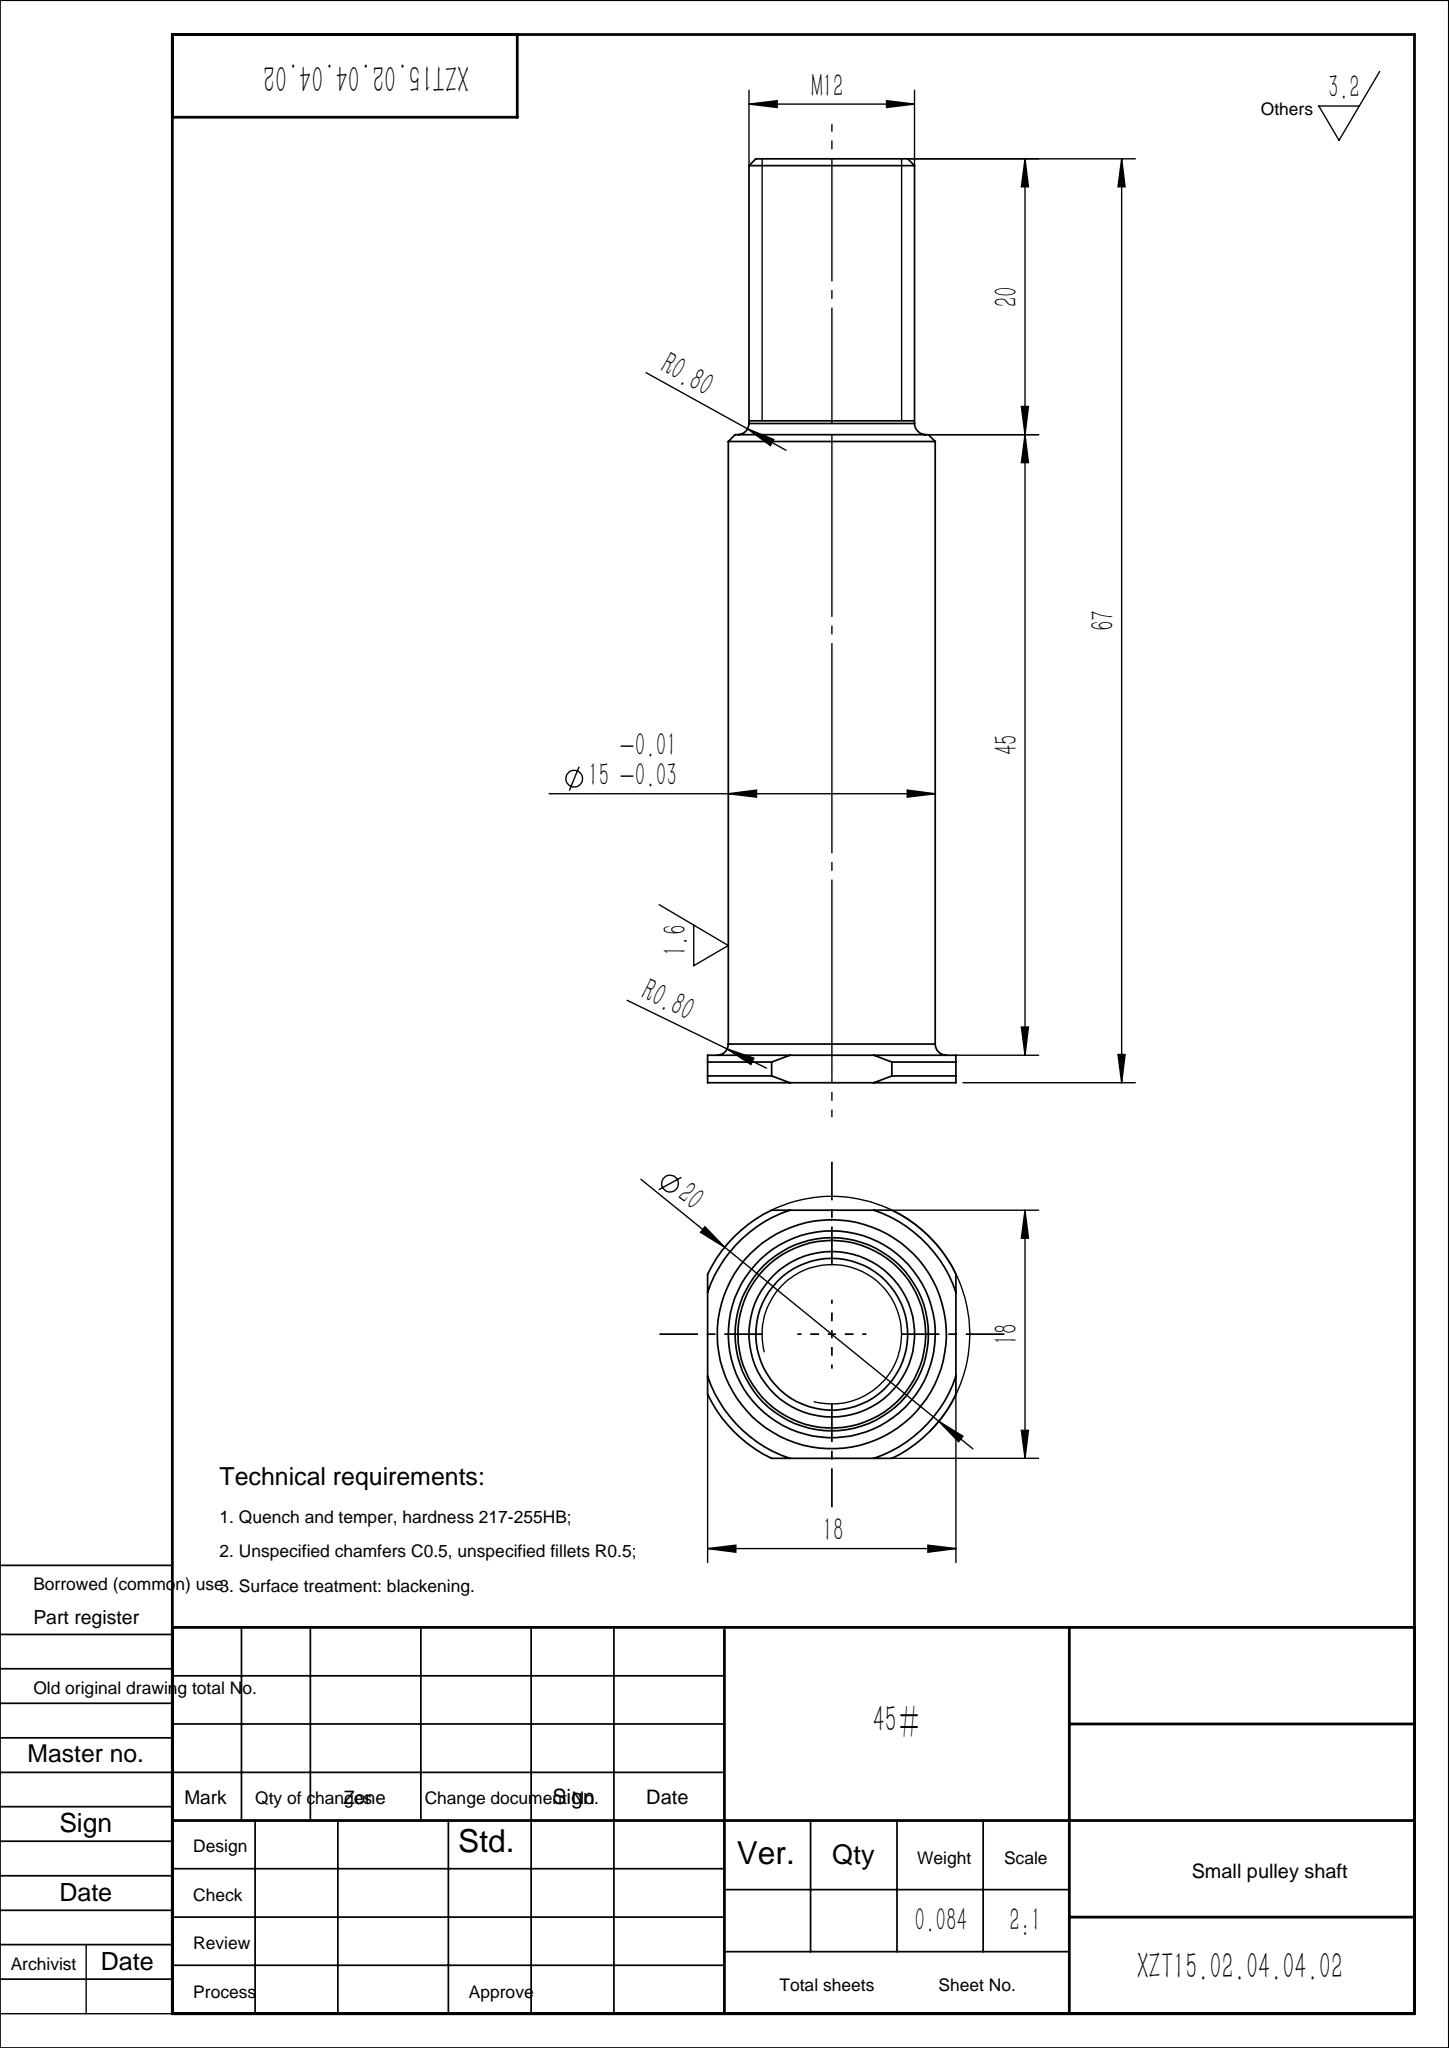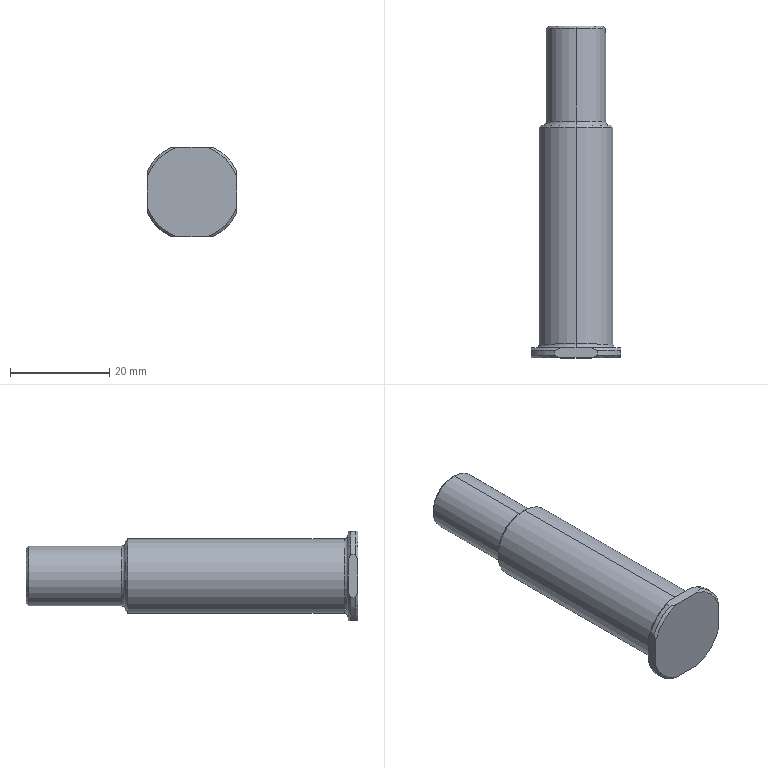Part | SolidWorks | features Chamfer 1, Fillet 1, ICE 1, Revolution 1 | 1 solid | 32 faces | box 18 x 67 x 18 mm | volume 10790 mm3 | cone 12 | cylinder 8 | plane 8 | torus 4 | commonest cylinder face diameters 20 x4 12 x2 15 x2
STEP:
#1=CARTESIAN_POINT('',(0.,2.,8.3));
#2=VERTEX_POINT('',#1);
#3=CARTESIAN_POINT('',(0.,2.,-8.3));
#4=VERTEX_POINT('',#3);
#5=CARTESIAN_POINT('',(0.,2.,0.));
#6=DIRECTION('',(0.,-1.,0.));
#7=DIRECTION('',(0.,0.,-1.));
#8=AXIS2_PLACEMENT_3D('',#5,#6,#7);
#9=CIRCLE('',#8,8.3);
#10=EDGE_CURVE('',#2,#4,#9,.T.);
#11=ORIENTED_EDGE('',*,*,#10,.F.);
#12=CARTESIAN_POINT('',(0.,2.8,7.5));
#13=VERTEX_POINT('',#12);
#14=CARTESIAN_POINT('',(0.,2.8,8.3));
#15=DIRECTION('',(1.,0.,0.));
#16=DIRECTION('',(0.,0.,-1.));
#17=AXIS2_PLACEMENT_3D('',#14,#15,#16);
#18=CIRCLE('',#17,0.8);
#19=EDGE_CURVE('',#2,#13,#18,.T.);
#20=ORIENTED_EDGE('',*,*,#19,.T.);
#21=CARTESIAN_POINT('',(0.,2.8,-7.5));
#22=VERTEX_POINT('',#21);
#23=CARTESIAN_POINT('',(0.,2.8,0.));
#24=DIRECTION('',(0.,1.,0.));
#25=DIRECTION('',(0.,0.,-1.));
#26=AXIS2_PLACEMENT_3D('',#23,#24,#25);
#27=CIRCLE('',#26,7.5);
#28=EDGE_CURVE('',#22,#13,#27,.T.);
#29=ORIENTED_EDGE('',*,*,#28,.F.);
#30=CARTESIAN_POINT('',(0.,2.8,-8.3));
#31=DIRECTION('',(-1.,0.,0.));
#32=DIRECTION('',(0.,0.,1.));
#33=AXIS2_PLACEMENT_3D('',#30,#31,#32);
#34=CIRCLE('',#33,0.8);
#35=EDGE_CURVE('',#4,#22,#34,.T.);
#36=ORIENTED_EDGE('',*,*,#35,.F.);
#37=EDGE_LOOP('',(#11,#20,#29,#36));
#38=FACE_OUTER_BOUND('',#37,.T.);
#39=CARTESIAN_POINT('',(0.,2.8,0.));
#40=DIRECTION('',(0.,-1.,0.));
#41=DIRECTION('',(0.,0.,-1.));
#42=AXIS2_PLACEMENT_3D('',#39,#40,#41);
#43=TOROIDAL_SURFACE('',#42,8.3,0.8);
#44=ADVANCED_FACE('',(#38),#43,.F.);
#45=CARTESIAN_POINT('',(0.,47.,6.8));
#46=VERTEX_POINT('',#45);
#47=CARTESIAN_POINT('',(0.,47.,-6.8));
#48=VERTEX_POINT('',#47);
#49=CARTESIAN_POINT('',(0.,47.,0.));
#50=DIRECTION('',(0.,-1.,0.));
#51=DIRECTION('',(0.,0.,-1.));
#52=AXIS2_PLACEMENT_3D('',#49,#50,#51);
#53=CIRCLE('',#52,6.8);
#54=EDGE_CURVE('',#46,#48,#53,.T.);
#55=ORIENTED_EDGE('',*,*,#54,.F.);
#56=CARTESIAN_POINT('',(0.,47.8,6.));
#57=VERTEX_POINT('',#56);
#58=CARTESIAN_POINT('',(0.,47.8,6.8));
#59=DIRECTION('',(1.,0.,0.));
#60=DIRECTION('',(0.,0.,-1.));
#61=AXIS2_PLACEMENT_3D('',#58,#59,#60);
#62=CIRCLE('',#61,0.8);
#63=EDGE_CURVE('',#46,#57,#62,.T.);
#64=ORIENTED_EDGE('',*,*,#63,.T.);
#65=CARTESIAN_POINT('',(0.,47.8,-6.));
#66=VERTEX_POINT('',#65);
#67=CARTESIAN_POINT('',(0.,47.8,0.));
#68=DIRECTION('',(0.,1.,0.));
#69=DIRECTION('',(0.,0.,-1.));
#70=AXIS2_PLACEMENT_3D('',#67,#68,#69);
#71=CIRCLE('',#70,6.);
#72=EDGE_CURVE('',#66,#57,#71,.T.);
#73=ORIENTED_EDGE('',*,*,#72,.F.);
#74=CARTESIAN_POINT('',(0.,47.8,-6.8));
#75=DIRECTION('',(-1.,0.,0.));
#76=DIRECTION('',(0.,0.,1.));
#77=AXIS2_PLACEMENT_3D('',#74,#75,#76);
#78=CIRCLE('',#77,0.8);
#79=EDGE_CURVE('',#48,#66,#78,.T.);
#80=ORIENTED_EDGE('',*,*,#79,.F.);
#81=EDGE_LOOP('',(#55,#64,#73,#80));
#82=FACE_OUTER_BOUND('',#81,.T.);
#83=CARTESIAN_POINT('',(0.,47.8,0.));
#84=DIRECTION('',(0.,-1.,0.));
#85=DIRECTION('',(0.,0.,-1.));
#86=AXIS2_PLACEMENT_3D('',#83,#84,#85);
#87=TOROIDAL_SURFACE('',#86,6.8,0.8);
#88=ADVANCED_FACE('',(#82),#87,.F.);
#89=CARTESIAN_POINT('',(0.,47.,7.));
#90=VERTEX_POINT('',#89);
#91=CARTESIAN_POINT('',(0.,47.,-7.));
#92=VERTEX_POINT('',#91);
#93=CARTESIAN_POINT('',(0.,47.,0.));
#94=DIRECTION('',(0.,1.,0.));
#95=DIRECTION('',(0.,0.,-1.));
#96=AXIS2_PLACEMENT_3D('',#93,#94,#95);
#97=CIRCLE('',#96,7.);
#98=EDGE_CURVE('',#90,#92,#97,.T.);
#99=ORIENTED_EDGE('',*,*,#98,.F.);
#100=CARTESIAN_POINT('',(0.,46.5,7.5));
#101=VERTEX_POINT('',#100);
#102=CARTESIAN_POINT('',(0.,47.,7.));
#103=DIRECTION('',(0.,-0.7071,0.7071));
#104=VECTOR('',#103,1000.);
#105=LINE('',#102,#104);
#106=EDGE_CURVE('',#90,#101,#105,.T.);
#107=ORIENTED_EDGE('',*,*,#106,.T.);
#108=CARTESIAN_POINT('',(0.,46.5,-7.5));
#109=VERTEX_POINT('',#108);
#110=CARTESIAN_POINT('',(0.,46.5,0.));
#111=DIRECTION('',(0.,-1.,0.));
#112=DIRECTION('',(0.,0.,-1.));
#113=AXIS2_PLACEMENT_3D('',#110,#111,#112);
#114=CIRCLE('',#113,7.5);
#115=EDGE_CURVE('',#109,#101,#114,.T.);
#116=ORIENTED_EDGE('',*,*,#115,.F.);
#117=CARTESIAN_POINT('',(0.,47.,-7.));
#118=DIRECTION('',(0.,-0.7071,-0.7071));
#119=VECTOR('',#118,1000.);
#120=LINE('',#117,#119);
#121=EDGE_CURVE('',#92,#109,#120,.T.);
#122=ORIENTED_EDGE('',*,*,#121,.F.);
#123=EDGE_LOOP('',(#99,#107,#116,#122));
#124=FACE_OUTER_BOUND('',#123,.T.);
#125=CARTESIAN_POINT('',(0.,47.,0.));
#126=DIRECTION('',(0.,-1.,0.));
#127=DIRECTION('',(0.,0.,-1.));
#128=AXIS2_PLACEMENT_3D('',#125,#126,#127);
#129=CONICAL_SURFACE('',#128,7.,0.7854);
#130=ADVANCED_FACE('',(#124),#129,.T.);
#131=CARTESIAN_POINT('',(0.,67.,5.5));
#132=VERTEX_POINT('',#131);
#133=CARTESIAN_POINT('',(0.,67.,-5.5));
#134=VERTEX_POINT('',#133);
#135=CARTESIAN_POINT('',(0.,67.,0.));
#136=DIRECTION('',(0.,1.,0.));
#137=DIRECTION('',(0.,0.,-1.));
#138=AXIS2_PLACEMENT_3D('',#135,#136,#137);
#139=CIRCLE('',#138,5.5);
#140=EDGE_CURVE('',#132,#134,#139,.T.);
#141=ORIENTED_EDGE('',*,*,#140,.F.);
#142=CARTESIAN_POINT('',(0.,66.5,6.));
#143=VERTEX_POINT('',#142);
#144=CARTESIAN_POINT('',(0.,67.,5.5));
#145=DIRECTION('',(0.,-0.7071,0.7071));
#146=VECTOR('',#145,1000.);
#147=LINE('',#144,#146);
#148=EDGE_CURVE('',#132,#143,#147,.T.);
#149=ORIENTED_EDGE('',*,*,#148,.T.);
#150=CARTESIAN_POINT('',(0.,66.5,-6.));
#151=VERTEX_POINT('',#150);
#152=CARTESIAN_POINT('',(0.,66.5,0.));
#153=DIRECTION('',(0.,-1.,0.));
#154=DIRECTION('',(0.,0.,-1.));
#155=AXIS2_PLACEMENT_3D('',#152,#153,#154);
#156=CIRCLE('',#155,6.);
#157=EDGE_CURVE('',#151,#143,#156,.T.);
#158=ORIENTED_EDGE('',*,*,#157,.F.);
#159=CARTESIAN_POINT('',(0.,67.,-5.5));
#160=DIRECTION('',(0.,-0.7071,-0.7071));
#161=VECTOR('',#160,1000.);
#162=LINE('',#159,#161);
#163=EDGE_CURVE('',#134,#151,#162,.T.);
#164=ORIENTED_EDGE('',*,*,#163,.F.);
#165=EDGE_LOOP('',(#141,#149,#158,#164));
#166=FACE_OUTER_BOUND('',#165,.T.);
#167=CARTESIAN_POINT('',(0.,67.,0.));
#168=DIRECTION('',(0.,-1.,0.));
#169=DIRECTION('',(0.,0.,-1.));
#170=AXIS2_PLACEMENT_3D('',#167,#168,#169);
#171=CONICAL_SURFACE('',#170,5.5,0.7854);
#172=ADVANCED_FACE('',(#166),#171,.T.);
#173=CARTESIAN_POINT('',(0.,47.8,0.));
#174=DIRECTION('',(0.,1.,0.));
#175=DIRECTION('',(0.,0.,-1.));
#176=AXIS2_PLACEMENT_3D('',#173,#174,#175);
#177=CIRCLE('',#176,6.);
#178=EDGE_CURVE('',#57,#66,#177,.T.);
#179=ORIENTED_EDGE('',*,*,#178,.T.);
#180=CARTESIAN_POINT('',(0.,0.,-6.));
#181=DIRECTION('',(0.,1.,0.));
#182=VECTOR('',#181,1000.);
#183=LINE('',#180,#182);
#184=EDGE_CURVE('',#66,#151,#183,.T.);
#185=ORIENTED_EDGE('',*,*,#184,.T.);
#186=ORIENTED_EDGE('',*,*,#157,.T.);
#187=CARTESIAN_POINT('',(0.,0.,6.));
#188=DIRECTION('',(0.,1.,0.));
#189=VECTOR('',#188,1000.);
#190=LINE('',#187,#189);
#191=EDGE_CURVE('',#57,#143,#190,.T.);
#192=ORIENTED_EDGE('',*,*,#191,.F.);
#193=EDGE_LOOP('',(#179,#185,#186,#192));
#194=FACE_OUTER_BOUND('',#193,.T.);
#195=CARTESIAN_POINT('',(0.,0.,0.));
#196=DIRECTION('',(0.,1.,0.));
#197=DIRECTION('',(0.,0.,1.));
#198=AXIS2_PLACEMENT_3D('',#195,#196,#197);
#199=CYLINDRICAL_SURFACE('',#198,6.);
#200=ADVANCED_FACE('',(#194),#199,.T.);
#201=CARTESIAN_POINT('',(0.,2.8,0.));
#202=DIRECTION('',(0.,1.,0.));
#203=DIRECTION('',(0.,0.,-1.));
#204=AXIS2_PLACEMENT_3D('',#201,#202,#203);
#205=CIRCLE('',#204,7.5);
#206=EDGE_CURVE('',#13,#22,#205,.T.);
#207=ORIENTED_EDGE('',*,*,#206,.T.);
#208=CARTESIAN_POINT('',(0.,0.,-7.5));
#209=DIRECTION('',(0.,1.,0.));
#210=VECTOR('',#209,1000.);
#211=LINE('',#208,#210);
#212=EDGE_CURVE('',#22,#109,#211,.T.);
#213=ORIENTED_EDGE('',*,*,#212,.T.);
#214=ORIENTED_EDGE('',*,*,#115,.T.);
#215=CARTESIAN_POINT('',(0.,0.,7.5));
#216=DIRECTION('',(0.,1.,0.));
#217=VECTOR('',#216,1000.);
#218=LINE('',#215,#217);
#219=EDGE_CURVE('',#13,#101,#218,.T.);
#220=ORIENTED_EDGE('',*,*,#219,.F.);
#221=EDGE_LOOP('',(#207,#213,#214,#220));
#222=FACE_OUTER_BOUND('',#221,.T.);
#223=CARTESIAN_POINT('',(0.,0.,0.));
#224=DIRECTION('',(0.,1.,0.));
#225=DIRECTION('',(0.,0.,1.));
#226=AXIS2_PLACEMENT_3D('',#223,#224,#225);
#227=CYLINDRICAL_SURFACE('',#226,7.5);
#228=ADVANCED_FACE('',(#222),#227,.T.);
#229=CARTESIAN_POINT('',(-4.359,0.5,-9.));
#230=VERTEX_POINT('',#229);
#231=CARTESIAN_POINT('',(-9.,0.5,-4.359));
#232=VERTEX_POINT('',#231);
#233=CARTESIAN_POINT('',(0.,0.5,0.));
#234=DIRECTION('',(0.,1.,0.));
#235=DIRECTION('',(0.,0.,1.));
#236=AXIS2_PLACEMENT_3D('',#233,#234,#235);
#237=CIRCLE('',#236,10.);
#238=EDGE_CURVE('',#230,#232,#237,.T.);
#239=ORIENTED_EDGE('',*,*,#238,.T.);
#240=CARTESIAN_POINT('',(-9.,1.5,-4.359));
#241=VERTEX_POINT('',#240);
#242=CARTESIAN_POINT('',(-9.,0.,-4.359));
#243=DIRECTION('',(0.,1.,0.));
#244=VECTOR('',#243,1000.);
#245=LINE('',#242,#244);
#246=EDGE_CURVE('',#232,#241,#245,.T.);
#247=ORIENTED_EDGE('',*,*,#246,.T.);
#248=CARTESIAN_POINT('',(-4.359,1.5,-9.));
#249=VERTEX_POINT('',#248);
#250=CARTESIAN_POINT('',(0.,1.5,0.));
#251=DIRECTION('',(0.,-1.,0.));
#252=DIRECTION('',(0.,0.,-1.));
#253=AXIS2_PLACEMENT_3D('',#250,#251,#252);
#254=CIRCLE('',#253,10.);
#255=EDGE_CURVE('',#241,#249,#254,.T.);
#256=ORIENTED_EDGE('',*,*,#255,.T.);
#257=CARTESIAN_POINT('',(-4.359,0.,-9.));
#258=DIRECTION('',(0.,-1.,0.));
#259=VECTOR('',#258,1000.);
#260=LINE('',#257,#259);
#261=EDGE_CURVE('',#249,#230,#260,.T.);
#262=ORIENTED_EDGE('',*,*,#261,.T.);
#263=EDGE_LOOP('',(#239,#247,#256,#262));
#264=FACE_OUTER_BOUND('',#263,.T.);
#265=CARTESIAN_POINT('',(0.,0.,0.));
#266=DIRECTION('',(0.,1.,0.));
#267=DIRECTION('',(0.,0.,1.));
#268=AXIS2_PLACEMENT_3D('',#265,#266,#267);
#269=CYLINDRICAL_SURFACE('',#268,10.);
#270=ADVANCED_FACE('',(#264),#269,.T.);
#271=CARTESIAN_POINT('',(-4.359,1.5,9.));
#272=VERTEX_POINT('',#271);
#273=CARTESIAN_POINT('',(-9.,1.5,4.359));
#274=VERTEX_POINT('',#273);
#275=CARTESIAN_POINT('',(0.,1.5,0.));
#276=DIRECTION('',(0.,-1.,0.));
#277=DIRECTION('',(0.,0.,-1.));
#278=AXIS2_PLACEMENT_3D('',#275,#276,#277);
#279=CIRCLE('',#278,10.);
#280=EDGE_CURVE('',#272,#274,#279,.T.);
#281=ORIENTED_EDGE('',*,*,#280,.T.);
#282=CARTESIAN_POINT('',(-9.,0.5,4.359));
#283=VERTEX_POINT('',#282);
#284=CARTESIAN_POINT('',(-9.,0.,4.359));
#285=DIRECTION('',(0.,-1.,0.));
#286=VECTOR('',#285,1000.);
#287=LINE('',#284,#286);
#288=EDGE_CURVE('',#274,#283,#287,.T.);
#289=ORIENTED_EDGE('',*,*,#288,.T.);
#290=CARTESIAN_POINT('',(-4.359,0.5,9.));
#291=VERTEX_POINT('',#290);
#292=CARTESIAN_POINT('',(0.,0.5,0.));
#293=DIRECTION('',(0.,1.,0.));
#294=DIRECTION('',(0.,0.,1.));
#295=AXIS2_PLACEMENT_3D('',#292,#293,#294);
#296=CIRCLE('',#295,10.);
#297=EDGE_CURVE('',#283,#291,#296,.T.);
#298=ORIENTED_EDGE('',*,*,#297,.T.);
#299=CARTESIAN_POINT('',(-4.359,0.,9.));
#300=DIRECTION('',(0.,1.,0.));
#301=VECTOR('',#300,1000.);
#302=LINE('',#299,#301);
#303=EDGE_CURVE('',#291,#272,#302,.T.);
#304=ORIENTED_EDGE('',*,*,#303,.T.);
#305=EDGE_LOOP('',(#281,#289,#298,#304));
#306=FACE_OUTER_BOUND('',#305,.T.);
#307=CARTESIAN_POINT('',(0.,0.,0.));
#308=DIRECTION('',(0.,1.,0.));
#309=DIRECTION('',(0.,0.,1.));
#310=AXIS2_PLACEMENT_3D('',#307,#308,#309);
#311=CYLINDRICAL_SURFACE('',#310,10.);
#312=ADVANCED_FACE('',(#306),#311,.T.);
#313=CARTESIAN_POINT('',(9.,1.5,4.359));
#314=VERTEX_POINT('',#313);
#315=CARTESIAN_POINT('',(4.359,1.5,9.));
#316=VERTEX_POINT('',#315);
#317=CARTESIAN_POINT('',(0.,1.5,0.));
#318=DIRECTION('',(0.,-1.,0.));
#319=DIRECTION('',(0.,0.,-1.));
#320=AXIS2_PLACEMENT_3D('',#317,#318,#319);
#321=CIRCLE('',#320,10.);
#322=EDGE_CURVE('',#314,#316,#321,.T.);
#323=ORIENTED_EDGE('',*,*,#322,.T.);
#324=CARTESIAN_POINT('',(4.359,0.5,9.));
#325=VERTEX_POINT('',#324);
#326=CARTESIAN_POINT('',(4.359,0.,9.));
#327=DIRECTION('',(0.,-1.,0.));
#328=VECTOR('',#327,1000.);
#329=LINE('',#326,#328);
#330=EDGE_CURVE('',#316,#325,#329,.T.);
#331=ORIENTED_EDGE('',*,*,#330,.T.);
#332=CARTESIAN_POINT('',(9.,0.5,4.359));
#333=VERTEX_POINT('',#332);
#334=CARTESIAN_POINT('',(0.,0.5,0.));
#335=DIRECTION('',(0.,1.,0.));
#336=DIRECTION('',(0.,0.,1.));
#337=AXIS2_PLACEMENT_3D('',#334,#335,#336);
#338=CIRCLE('',#337,10.);
#339=EDGE_CURVE('',#325,#333,#338,.T.);
#340=ORIENTED_EDGE('',*,*,#339,.T.);
#341=CARTESIAN_POINT('',(9.,0.,4.359));
#342=DIRECTION('',(0.,1.,0.));
#343=VECTOR('',#342,1000.);
#344=LINE('',#341,#343);
#345=EDGE_CURVE('',#333,#314,#344,.T.);
#346=ORIENTED_EDGE('',*,*,#345,.T.);
#347=EDGE_LOOP('',(#323,#331,#340,#346));
#348=FACE_OUTER_BOUND('',#347,.T.);
#349=CARTESIAN_POINT('',(0.,0.,0.));
#350=DIRECTION('',(0.,1.,0.));
#351=DIRECTION('',(0.,0.,1.));
#352=AXIS2_PLACEMENT_3D('',#349,#350,#351);
#353=CYLINDRICAL_SURFACE('',#352,10.);
#354=ADVANCED_FACE('',(#348),#353,.T.);
#355=CARTESIAN_POINT('',(-9.,2.,3.041));
#356=VERTEX_POINT('',#355);
#357=CARTESIAN_POINT('',(-9.,1.5,4.359));
#358=CARTESIAN_POINT('',(-9.,1.688,3.928));
#359=CARTESIAN_POINT('',(-9.,1.857,3.489));
#360=CARTESIAN_POINT('',(-9.,2.,3.041));
#361=B_SPLINE_CURVE_WITH_KNOTS('',3,(#357,#358,#359,#360),.UNSPECIFIED.,.F.,.F.,(4,4),(0.01807,0.01948),.UNSPECIFIED.);
#362=EDGE_CURVE('',#274,#356,#361,.T.);
#363=ORIENTED_EDGE('',*,*,#362,.F.);
#364=ORIENTED_EDGE('',*,*,#280,.F.);
#365=CARTESIAN_POINT('',(-3.041,2.,9.));
#366=VERTEX_POINT('',#365);
#367=CARTESIAN_POINT('',(-3.041,2.,9.));
#368=CARTESIAN_POINT('',(-3.488,1.857,9.));
#369=CARTESIAN_POINT('',(-3.927,1.688,9.));
#370=CARTESIAN_POINT('',(-4.359,1.5,9.));
#371=B_SPLINE_CURVE_WITH_KNOTS('',3,(#367,#368,#369,#370),.UNSPECIFIED.,.F.,.F.,(4,4),(0.02566,0.02708),.UNSPECIFIED.);
#372=EDGE_CURVE('',#366,#272,#371,.T.);
#373=ORIENTED_EDGE('',*,*,#372,.F.);
#374=CARTESIAN_POINT('',(0.,2.,0.));
#375=DIRECTION('',(0.,1.,0.));
#376=DIRECTION('',(0.,0.,-1.));
#377=AXIS2_PLACEMENT_3D('',#374,#375,#376);
#378=CIRCLE('',#377,9.5);
#379=EDGE_CURVE('',#356,#366,#378,.T.);
#380=ORIENTED_EDGE('',*,*,#379,.F.);
#381=EDGE_LOOP('',(#363,#364,#373,#380));
#382=FACE_OUTER_BOUND('',#381,.T.);
#383=CARTESIAN_POINT('',(0.,2.,0.));
#384=DIRECTION('',(0.,-1.,0.));
#385=DIRECTION('',(0.,0.,-1.));
#386=AXIS2_PLACEMENT_3D('',#383,#384,#385);
#387=CONICAL_SURFACE('',#386,9.5,0.7854);
#388=ADVANCED_FACE('',(#382),#387,.T.);
#389=CARTESIAN_POINT('',(3.041,2.,9.));
#390=VERTEX_POINT('',#389);
#391=CARTESIAN_POINT('',(4.359,1.5,9.));
#392=CARTESIAN_POINT('',(3.928,1.688,9.));
#393=CARTESIAN_POINT('',(3.489,1.857,9.));
#394=CARTESIAN_POINT('',(3.041,2.,9.));
#395=B_SPLINE_CURVE_WITH_KNOTS('',3,(#391,#392,#393,#394),.UNSPECIFIED.,.F.,.F.,(4,4),(0.01807,0.01948),.UNSPECIFIED.);
#396=EDGE_CURVE('',#316,#390,#395,.T.);
#397=ORIENTED_EDGE('',*,*,#396,.F.);
#398=ORIENTED_EDGE('',*,*,#322,.F.);
#399=CARTESIAN_POINT('',(9.,2.,3.041));
#400=VERTEX_POINT('',#399);
#401=CARTESIAN_POINT('',(9.,2.,3.041));
#402=CARTESIAN_POINT('',(9.,1.857,3.488));
#403=CARTESIAN_POINT('',(9.,1.688,3.927));
#404=CARTESIAN_POINT('',(9.,1.5,4.359));
#405=B_SPLINE_CURVE_WITH_KNOTS('',3,(#401,#402,#403,#404),.UNSPECIFIED.,.F.,.F.,(4,4),(0.02566,0.02708),.UNSPECIFIED.);
#406=EDGE_CURVE('',#400,#314,#405,.T.);
#407=ORIENTED_EDGE('',*,*,#406,.F.);
#408=CARTESIAN_POINT('',(0.,2.,0.));
#409=DIRECTION('',(0.,1.,0.));
#410=DIRECTION('',(0.,0.,-1.));
#411=AXIS2_PLACEMENT_3D('',#408,#409,#410);
#412=CIRCLE('',#411,9.5);
#413=EDGE_CURVE('',#390,#400,#412,.T.);
#414=ORIENTED_EDGE('',*,*,#413,.F.);
#415=EDGE_LOOP('',(#397,#398,#407,#414));
#416=FACE_OUTER_BOUND('',#415,.T.);
#417=CARTESIAN_POINT('',(0.,2.,0.));
#418=DIRECTION('',(0.,-1.,0.));
#419=DIRECTION('',(0.,0.,-1.));
#420=AXIS2_PLACEMENT_3D('',#417,#418,#419);
#421=CONICAL_SURFACE('',#420,9.5,0.7854);
#422=ADVANCED_FACE('',(#416),#421,.T.);
#423=CARTESIAN_POINT('',(9.,1.5,-4.359));
#424=VERTEX_POINT('',#423);
#425=CARTESIAN_POINT('',(9.,2.,-3.041));
#426=VERTEX_POINT('',#425);
#427=CARTESIAN_POINT('',(9.,1.5,-4.359));
#428=CARTESIAN_POINT('',(9.,1.688,-3.928));
#429=CARTESIAN_POINT('',(9.,1.857,-3.489));
#430=CARTESIAN_POINT('',(9.,2.,-3.041));
#431=B_SPLINE_CURVE_WITH_KNOTS('',3,(#427,#428,#429,#430),.UNSPECIFIED.,.F.,.F.,(4,4),(0.01807,0.01948),.UNSPECIFIED.);
#432=EDGE_CURVE('',#424,#426,#431,.T.);
#433=ORIENTED_EDGE('',*,*,#432,.F.);
#434=CARTESIAN_POINT('',(4.359,1.5,-9.));
#435=VERTEX_POINT('',#434);
#436=CARTESIAN_POINT('',(0.,1.5,0.));
#437=DIRECTION('',(0.,-1.,0.));
#438=DIRECTION('',(0.,0.,-1.));
#439=AXIS2_PLACEMENT_3D('',#436,#437,#438);
#440=CIRCLE('',#439,10.);
#441=EDGE_CURVE('',#435,#424,#440,.T.);
#442=ORIENTED_EDGE('',*,*,#441,.F.);
#443=CARTESIAN_POINT('',(3.041,2.,-9.));
#444=VERTEX_POINT('',#443);
#445=CARTESIAN_POINT('',(3.041,2.,-9.));
#446=CARTESIAN_POINT('',(3.488,1.857,-9.));
#447=CARTESIAN_POINT('',(3.927,1.688,-9.));
#448=CARTESIAN_POINT('',(4.359,1.5,-9.));
#449=B_SPLINE_CURVE_WITH_KNOTS('',3,(#445,#446,#447,#448),.UNSPECIFIED.,.F.,.F.,(4,4),(0.02566,0.02708),.UNSPECIFIED.);
#450=EDGE_CURVE('',#444,#435,#449,.T.);
#451=ORIENTED_EDGE('',*,*,#450,.F.);
#452=CARTESIAN_POINT('',(0.,2.,0.));
#453=DIRECTION('',(0.,1.,0.));
#454=DIRECTION('',(0.,0.,-1.));
#455=AXIS2_PLACEMENT_3D('',#452,#453,#454);
#456=CIRCLE('',#455,9.5);
#457=EDGE_CURVE('',#426,#444,#456,.T.);
#458=ORIENTED_EDGE('',*,*,#457,.F.);
#459=EDGE_LOOP('',(#433,#442,#451,#458));
#460=FACE_OUTER_BOUND('',#459,.T.);
#461=CARTESIAN_POINT('',(0.,2.,0.));
#462=DIRECTION('',(0.,-1.,0.));
#463=DIRECTION('',(0.,0.,-1.));
#464=AXIS2_PLACEMENT_3D('',#461,#462,#463);
#465=CONICAL_SURFACE('',#464,9.5,0.7854);
#466=ADVANCED_FACE('',(#460),#465,.T.);
#467=CARTESIAN_POINT('',(-9.,0.,-3.041));
#468=VERTEX_POINT('',#467);
#469=CARTESIAN_POINT('',(-9.,0.5,-4.359));
#470=CARTESIAN_POINT('',(-9.,0.312,-3.928));
#471=CARTESIAN_POINT('',(-9.,0.1434,-3.489));
#472=CARTESIAN_POINT('',(-9.,0.,-3.041));
#473=B_SPLINE_CURVE_WITH_KNOTS('',3,(#469,#470,#471,#472),.UNSPECIFIED.,.F.,.F.,(4,4),(0.01807,0.01948),.UNSPECIFIED.);
#474=EDGE_CURVE('',#232,#468,#473,.T.);
#475=ORIENTED_EDGE('',*,*,#474,.F.);
#476=ORIENTED_EDGE('',*,*,#238,.F.);
#477=CARTESIAN_POINT('',(-3.041,0.,-9.));
#478=VERTEX_POINT('',#477);
#479=CARTESIAN_POINT('',(-3.041,0.,-9.));
#480=CARTESIAN_POINT('',(-3.488,0.1431,-9.));
#481=CARTESIAN_POINT('',(-3.927,0.3117,-9.));
#482=CARTESIAN_POINT('',(-4.359,0.5,-9.));
#483=B_SPLINE_CURVE_WITH_KNOTS('',3,(#479,#480,#481,#482),.UNSPECIFIED.,.F.,.F.,(4,4),(0.02566,0.02708),.UNSPECIFIED.);
#484=EDGE_CURVE('',#478,#230,#483,.T.);
#485=ORIENTED_EDGE('',*,*,#484,.F.);
#486=CARTESIAN_POINT('',(0.,0.,0.));
#487=DIRECTION('',(0.,-1.,0.));
#488=DIRECTION('',(0.,0.,1.));
#489=AXIS2_PLACEMENT_3D('',#486,#487,#488);
#490=CIRCLE('',#489,9.5);
#491=EDGE_CURVE('',#468,#478,#490,.T.);
#492=ORIENTED_EDGE('',*,*,#491,.F.);
#493=EDGE_LOOP('',(#475,#476,#485,#492));
#494=FACE_OUTER_BOUND('',#493,.T.);
#495=CARTESIAN_POINT('',(0.,0.5,0.));
#496=DIRECTION('',(0.,1.,0.));
#497=DIRECTION('',(0.,0.,1.));
#498=AXIS2_PLACEMENT_3D('',#495,#496,#497);
#499=CONICAL_SURFACE('',#498,10.,0.7854);
#500=ADVANCED_FACE('',(#494),#499,.T.);
#501=CARTESIAN_POINT('',(-9.,0.,3.041));
#502=VERTEX_POINT('',#501);
#503=CARTESIAN_POINT('',(-9.,0.,3.041));
#504=CARTESIAN_POINT('',(-9.,0.1431,3.488));
#505=CARTESIAN_POINT('',(-9.,0.3117,3.927));
#506=CARTESIAN_POINT('',(-9.,0.5,4.359));
#507=B_SPLINE_CURVE_WITH_KNOTS('',3,(#503,#504,#505,#506),.UNSPECIFIED.,.F.,.F.,(4,4),(0.02566,0.02708),.UNSPECIFIED.);
#508=EDGE_CURVE('',#502,#283,#507,.T.);
#509=ORIENTED_EDGE('',*,*,#508,.F.);
#510=CARTESIAN_POINT('',(-3.041,0.,9.));
#511=VERTEX_POINT('',#510);
#512=CARTESIAN_POINT('',(0.,0.,0.));
#513=DIRECTION('',(0.,-1.,0.));
#514=DIRECTION('',(0.,0.,1.));
#515=AXIS2_PLACEMENT_3D('',#512,#513,#514);
#516=CIRCLE('',#515,9.5);
#517=EDGE_CURVE('',#511,#502,#516,.T.);
#518=ORIENTED_EDGE('',*,*,#517,.F.);
#519=CARTESIAN_POINT('',(-4.359,0.5,9.));
#520=CARTESIAN_POINT('',(-3.928,0.312,9.));
#521=CARTESIAN_POINT('',(-3.489,0.1434,9.));
#522=CARTESIAN_POINT('',(-3.041,0.,9.));
#523=B_SPLINE_CURVE_WITH_KNOTS('',3,(#519,#520,#521,#522),.UNSPECIFIED.,.F.,.F.,(4,4),(0.01807,0.01948),.UNSPECIFIED.);
#524=EDGE_CURVE('',#291,#511,#523,.T.);
#525=ORIENTED_EDGE('',*,*,#524,.F.);
#526=ORIENTED_EDGE('',*,*,#297,.F.);
#527=EDGE_LOOP('',(#509,#518,#525,#526));
#528=FACE_OUTER_BOUND('',#527,.T.);
#529=CARTESIAN_POINT('',(0.,0.5,0.));
#530=DIRECTION('',(0.,1.,0.));
#531=DIRECTION('',(0.,0.,1.));
#532=AXIS2_PLACEMENT_3D('',#529,#530,#531);
#533=CONICAL_SURFACE('',#532,10.,0.7854);
#534=ADVANCED_FACE('',(#528),#533,.T.);
#535=CARTESIAN_POINT('',(3.041,0.,9.));
#536=VERTEX_POINT('',#535);
#537=CARTESIAN_POINT('',(3.041,0.,9.));
#538=CARTESIAN_POINT('',(3.488,0.1431,9.));
#539=CARTESIAN_POINT('',(3.927,0.3117,9.));
#540=CARTESIAN_POINT('',(4.359,0.5,9.));
#541=B_SPLINE_CURVE_WITH_KNOTS('',3,(#537,#538,#539,#540),.UNSPECIFIED.,.F.,.F.,(4,4),(0.02566,0.02708),.UNSPECIFIED.);
#542=EDGE_CURVE('',#536,#325,#541,.T.);
#543=ORIENTED_EDGE('',*,*,#542,.F.);
#544=CARTESIAN_POINT('',(9.,0.,3.041));
#545=VERTEX_POINT('',#544);
#546=CARTESIAN_POINT('',(0.,0.,0.));
#547=DIRECTION('',(0.,-1.,0.));
#548=DIRECTION('',(0.,0.,1.));
#549=AXIS2_PLACEMENT_3D('',#546,#547,#548);
#550=CIRCLE('',#549,9.5);
#551=EDGE_CURVE('',#545,#536,#550,.T.);
#552=ORIENTED_EDGE('',*,*,#551,.F.);
#553=CARTESIAN_POINT('',(9.,0.5,4.359));
#554=CARTESIAN_POINT('',(9.,0.312,3.928));
#555=CARTESIAN_POINT('',(9.,0.1434,3.489));
#556=CARTESIAN_POINT('',(9.,0.,3.041));
#557=B_SPLINE_CURVE_WITH_KNOTS('',3,(#553,#554,#555,#556),.UNSPECIFIED.,.F.,.F.,(4,4),(0.01807,0.01948),.UNSPECIFIED.);
#558=EDGE_CURVE('',#333,#545,#557,.T.);
#559=ORIENTED_EDGE('',*,*,#558,.F.);
#560=ORIENTED_EDGE('',*,*,#339,.F.);
#561=EDGE_LOOP('',(#543,#552,#559,#560));
#562=FACE_OUTER_BOUND('',#561,.T.);
#563=CARTESIAN_POINT('',(0.,0.5,0.));
#564=DIRECTION('',(0.,1.,0.));
#565=DIRECTION('',(0.,0.,1.));
#566=AXIS2_PLACEMENT_3D('',#563,#564,#565);
#567=CONICAL_SURFACE('',#566,10.,0.7854);
#568=ADVANCED_FACE('',(#562),#567,.T.);
#569=ORIENTED_EDGE('',*,*,#517,.T.);
#570=CARTESIAN_POINT('',(-9.,0.,9.));
#571=DIRECTION('',(0.,0.,1.));
#572=VECTOR('',#571,1000.);
#573=LINE('',#570,#572);
#574=EDGE_CURVE('',#468,#502,#573,.T.);
#575=ORIENTED_EDGE('',*,*,#574,.F.);
#576=ORIENTED_EDGE('',*,*,#491,.T.);
#577=CARTESIAN_POINT('',(3.041,0.,-9.));
#578=VERTEX_POINT('',#577);
#579=CARTESIAN_POINT('',(9.,0.,-9.));
#580=DIRECTION('',(-1.,0.,0.));
#581=VECTOR('',#580,1000.);
#582=LINE('',#579,#581);
#583=EDGE_CURVE('',#578,#478,#582,.T.);
#584=ORIENTED_EDGE('',*,*,#583,.F.);
#585=CARTESIAN_POINT('',(9.,0.,-3.041));
#586=VERTEX_POINT('',#585);
#587=CARTESIAN_POINT('',(0.,0.,0.));
#588=DIRECTION('',(0.,-1.,0.));
#589=DIRECTION('',(0.,0.,1.));
#590=AXIS2_PLACEMENT_3D('',#587,#588,#589);
#591=CIRCLE('',#590,9.5);
#592=EDGE_CURVE('',#578,#586,#591,.T.);
#593=ORIENTED_EDGE('',*,*,#592,.T.);
#594=CARTESIAN_POINT('',(9.,0.,9.));
#595=DIRECTION('',(0.,0.,-1.));
#596=VECTOR('',#595,1000.);
#597=LINE('',#594,#596);
#598=EDGE_CURVE('',#545,#586,#597,.T.);
#599=ORIENTED_EDGE('',*,*,#598,.F.);
#600=ORIENTED_EDGE('',*,*,#551,.T.);
#601=CARTESIAN_POINT('',(9.,0.,9.));
#602=DIRECTION('',(1.,0.,0.));
#603=VECTOR('',#602,1000.);
#604=LINE('',#601,#603);
#605=EDGE_CURVE('',#511,#536,#604,.T.);
#606=ORIENTED_EDGE('',*,*,#605,.F.);
#607=EDGE_LOOP('',(#569,#575,#576,#584,#593,#599,#600,#606));
#608=FACE_OUTER_BOUND('',#607,.T.);
#609=CARTESIAN_POINT('',(0.,0.,0.));
#610=DIRECTION('',(0.,1.,0.));
#611=DIRECTION('',(0.,0.,1.));
#612=AXIS2_PLACEMENT_3D('',#609,#610,#611);
#613=PLANE('',#612);
#614=ADVANCED_FACE('',(#608),#613,.F.);
#615=ORIENTED_EDGE('',*,*,#441,.T.);
#616=CARTESIAN_POINT('',(9.,0.5,-4.359));
#617=VERTEX_POINT('',#616);
#618=CARTESIAN_POINT('',(9.,0.,-4.359));
#619=DIRECTION('',(0.,-1.,0.));
#620=VECTOR('',#619,1000.);
#621=LINE('',#618,#620);
#622=EDGE_CURVE('',#424,#617,#621,.T.);
#623=ORIENTED_EDGE('',*,*,#622,.T.);
#624=CARTESIAN_POINT('',(4.359,0.5,-9.));
#625=VERTEX_POINT('',#624);
#626=CARTESIAN_POINT('',(0.,0.5,0.));
#627=DIRECTION('',(0.,1.,0.));
#628=DIRECTION('',(0.,0.,1.));
#629=AXIS2_PLACEMENT_3D('',#626,#627,#628);
#630=CIRCLE('',#629,10.);
#631=EDGE_CURVE('',#617,#625,#630,.T.);
#632=ORIENTED_EDGE('',*,*,#631,.T.);
#633=CARTESIAN_POINT('',(4.359,0.,-9.));
#634=DIRECTION('',(0.,1.,0.));
#635=VECTOR('',#634,1000.);
#636=LINE('',#633,#635);
#637=EDGE_CURVE('',#625,#435,#636,.T.);
#638=ORIENTED_EDGE('',*,*,#637,.T.);
#639=EDGE_LOOP('',(#615,#623,#632,#638));
#640=FACE_OUTER_BOUND('',#639,.T.);
#641=CARTESIAN_POINT('',(0.,0.,0.));
#642=DIRECTION('',(0.,1.,0.));
#643=DIRECTION('',(0.,0.,1.));
#644=AXIS2_PLACEMENT_3D('',#641,#642,#643);
#645=CYLINDRICAL_SURFACE('',#644,10.);
#646=ADVANCED_FACE('',(#640),#645,.T.);
#647=CARTESIAN_POINT('',(0.,2.,0.));
#648=DIRECTION('',(0.,-1.,0.));
#649=DIRECTION('',(0.,0.,-1.));
#650=AXIS2_PLACEMENT_3D('',#647,#648,#649);
#651=CIRCLE('',#650,8.3);
#652=EDGE_CURVE('',#4,#2,#651,.T.);
#653=ORIENTED_EDGE('',*,*,#652,.T.);
#654=ORIENTED_EDGE('',*,*,#10,.T.);
#655=EDGE_LOOP('',(#653,#654));
#656=FACE_BOUND('',#655,.T.);
#657=CARTESIAN_POINT('',(-3.041,2.,-9.));
#658=VERTEX_POINT('',#657);
#659=CARTESIAN_POINT('',(-9.,2.,-3.041));
#660=VERTEX_POINT('',#659);
#661=CARTESIAN_POINT('',(0.,2.,0.));
#662=DIRECTION('',(0.,1.,0.));
#663=DIRECTION('',(0.,0.,-1.));
#664=AXIS2_PLACEMENT_3D('',#661,#662,#663);
#665=CIRCLE('',#664,9.5);
#666=EDGE_CURVE('',#658,#660,#665,.T.);
#667=ORIENTED_EDGE('',*,*,#666,.T.);
#668=CARTESIAN_POINT('',(-9.,2.,0.));
#669=DIRECTION('',(0.,0.,1.));
#670=VECTOR('',#669,1000.);
#671=LINE('',#668,#670);
#672=EDGE_CURVE('',#660,#356,#671,.T.);
#673=ORIENTED_EDGE('',*,*,#672,.T.);
#674=ORIENTED_EDGE('',*,*,#379,.T.);
#675=CARTESIAN_POINT('',(10.,2.,9.));
#676=DIRECTION('',(1.,0.,0.));
#677=VECTOR('',#676,1000.);
#678=LINE('',#675,#677);
#679=EDGE_CURVE('',#366,#390,#678,.T.);
#680=ORIENTED_EDGE('',*,*,#679,.T.);
#681=ORIENTED_EDGE('',*,*,#413,.T.);
#682=CARTESIAN_POINT('',(9.,2.,0.));
#683=DIRECTION('',(0.,0.,-1.));
#684=VECTOR('',#683,1000.);
#685=LINE('',#682,#684);
#686=EDGE_CURVE('',#400,#426,#685,.T.);
#687=ORIENTED_EDGE('',*,*,#686,.T.);
#688=ORIENTED_EDGE('',*,*,#457,.T.);
#689=CARTESIAN_POINT('',(10.,2.,-9.));
#690=DIRECTION('',(-1.,0.,0.));
#691=VECTOR('',#690,1000.);
#692=LINE('',#689,#691);
#693=EDGE_CURVE('',#444,#658,#692,.T.);
#694=ORIENTED_EDGE('',*,*,#693,.T.);
#695=EDGE_LOOP('',(#667,#673,#674,#680,#681,#687,#688,#694));
#696=FACE_OUTER_BOUND('',#695,.T.);
#697=CARTESIAN_POINT('',(10.,2.,0.));
#698=DIRECTION('',(0.,-1.,0.));
#699=DIRECTION('',(0.,0.,-1.));
#700=AXIS2_PLACEMENT_3D('',#697,#698,#699);
#701=PLANE('',#700);
#702=ADVANCED_FACE('',(#656,#696),#701,.F.);
#703=ORIENTED_EDGE('',*,*,#212,.F.);
#704=ORIENTED_EDGE('',*,*,#28,.T.);
#705=ORIENTED_EDGE('',*,*,#219,.T.);
#706=CARTESIAN_POINT('',(0.,46.5,0.));
#707=DIRECTION('',(0.,-1.,0.));
#708=DIRECTION('',(0.,0.,-1.));
#709=AXIS2_PLACEMENT_3D('',#706,#707,#708);
#710=CIRCLE('',#709,7.5);
#711=EDGE_CURVE('',#101,#109,#710,.T.);
#712=ORIENTED_EDGE('',*,*,#711,.T.);
#713=EDGE_LOOP('',(#703,#704,#705,#712));
#714=FACE_OUTER_BOUND('',#713,.T.);
#715=CARTESIAN_POINT('',(0.,0.,0.));
#716=DIRECTION('',(0.,1.,0.));
#717=DIRECTION('',(0.,0.,1.));
#718=AXIS2_PLACEMENT_3D('',#715,#716,#717);
#719=CYLINDRICAL_SURFACE('',#718,7.5);
#720=ADVANCED_FACE('',(#714),#719,.T.);
#721=CARTESIAN_POINT('',(0.,47.,0.));
#722=DIRECTION('',(0.,-1.,0.));
#723=DIRECTION('',(0.,0.,-1.));
#724=AXIS2_PLACEMENT_3D('',#721,#722,#723);
#725=CIRCLE('',#724,6.8);
#726=EDGE_CURVE('',#48,#46,#725,.T.);
#727=ORIENTED_EDGE('',*,*,#726,.T.);
#728=ORIENTED_EDGE('',*,*,#54,.T.);
#729=EDGE_LOOP('',(#727,#728));
#730=FACE_BOUND('',#729,.T.);
#731=CARTESIAN_POINT('',(0.,47.,0.));
#732=DIRECTION('',(0.,1.,0.));
#733=DIRECTION('',(0.,0.,-1.));
#734=AXIS2_PLACEMENT_3D('',#731,#732,#733);
#735=CIRCLE('',#734,7.);
#736=EDGE_CURVE('',#92,#90,#735,.T.);
#737=ORIENTED_EDGE('',*,*,#736,.T.);
#738=ORIENTED_EDGE('',*,*,#98,.T.);
#739=EDGE_LOOP('',(#737,#738));
#740=FACE_OUTER_BOUND('',#739,.T.);
#741=CARTESIAN_POINT('',(7.5,47.,0.));
#742=DIRECTION('',(0.,-1.,0.));
#743=DIRECTION('',(0.,0.,-1.));
#744=AXIS2_PLACEMENT_3D('',#741,#742,#743);
#745=PLANE('',#744);
#746=ADVANCED_FACE('',(#730,#740),#745,.F.);
#747=ORIENTED_EDGE('',*,*,#184,.F.);
#748=ORIENTED_EDGE('',*,*,#72,.T.);
#749=ORIENTED_EDGE('',*,*,#191,.T.);
#750=CARTESIAN_POINT('',(0.,66.5,0.));
#751=DIRECTION('',(0.,-1.,0.));
#752=DIRECTION('',(0.,0.,-1.));
#753=AXIS2_PLACEMENT_3D('',#750,#751,#752);
#754=CIRCLE('',#753,6.);
#755=EDGE_CURVE('',#143,#151,#754,.T.);
#756=ORIENTED_EDGE('',*,*,#755,.T.);
#757=EDGE_LOOP('',(#747,#748,#749,#756));
#758=FACE_OUTER_BOUND('',#757,.T.);
#759=CARTESIAN_POINT('',(0.,0.,0.));
#760=DIRECTION('',(0.,1.,0.));
#761=DIRECTION('',(0.,0.,1.));
#762=AXIS2_PLACEMENT_3D('',#759,#760,#761);
#763=CYLINDRICAL_SURFACE('',#762,6.);
#764=ADVANCED_FACE('',(#758),#763,.T.);
#765=CARTESIAN_POINT('',(0.,67.,0.));
#766=DIRECTION('',(0.,1.,0.));
#767=DIRECTION('',(0.,0.,-1.));
#768=AXIS2_PLACEMENT_3D('',#765,#766,#767);
#769=CIRCLE('',#768,5.5);
#770=EDGE_CURVE('',#134,#132,#769,.T.);
#771=ORIENTED_EDGE('',*,*,#770,.T.);
#772=ORIENTED_EDGE('',*,*,#140,.T.);
#773=EDGE_LOOP('',(#771,#772));
#774=FACE_OUTER_BOUND('',#773,.T.);
#775=CARTESIAN_POINT('',(6.,67.,0.));
#776=DIRECTION('',(0.,-1.,0.));
#777=DIRECTION('',(0.,0.,-1.));
#778=AXIS2_PLACEMENT_3D('',#775,#776,#777);
#779=PLANE('',#778);
#780=ADVANCED_FACE('',(#774),#779,.F.);
#781=ORIENTED_EDGE('',*,*,#148,.F.);
#782=ORIENTED_EDGE('',*,*,#770,.F.);
#783=ORIENTED_EDGE('',*,*,#163,.T.);
#784=ORIENTED_EDGE('',*,*,#755,.F.);
#785=EDGE_LOOP('',(#781,#782,#783,#784));
#786=FACE_OUTER_BOUND('',#785,.T.);
#787=CARTESIAN_POINT('',(0.,67.,0.));
#788=DIRECTION('',(0.,-1.,0.));
#789=DIRECTION('',(0.,0.,-1.));
#790=AXIS2_PLACEMENT_3D('',#787,#788,#789);
#791=CONICAL_SURFACE('',#790,5.5,0.7854);
#792=ADVANCED_FACE('',(#786),#791,.T.);
#793=CARTESIAN_POINT('',(-9.,2.,-3.041));
#794=CARTESIAN_POINT('',(-9.,1.857,-3.488));
#795=CARTESIAN_POINT('',(-9.,1.688,-3.927));
#796=CARTESIAN_POINT('',(-9.,1.5,-4.359));
#797=B_SPLINE_CURVE_WITH_KNOTS('',3,(#793,#794,#795,#796),.UNSPECIFIED.,.F.,.F.,(4,4),(0.02566,0.02708),.UNSPECIFIED.);
#798=EDGE_CURVE('',#660,#241,#797,.T.);
#799=ORIENTED_EDGE('',*,*,#798,.F.);
#800=ORIENTED_EDGE('',*,*,#666,.F.);
#801=CARTESIAN_POINT('',(-4.359,1.5,-9.));
#802=CARTESIAN_POINT('',(-3.928,1.688,-9.));
#803=CARTESIAN_POINT('',(-3.489,1.857,-9.));
#804=CARTESIAN_POINT('',(-3.041,2.,-9.));
#805=B_SPLINE_CURVE_WITH_KNOTS('',3,(#801,#802,#803,#804),.UNSPECIFIED.,.F.,.F.,(4,4),(0.01807,0.01948),.UNSPECIFIED.);
#806=EDGE_CURVE('',#249,#658,#805,.T.);
#807=ORIENTED_EDGE('',*,*,#806,.F.);
#808=ORIENTED_EDGE('',*,*,#255,.F.);
#809=EDGE_LOOP('',(#799,#800,#807,#808));
#810=FACE_OUTER_BOUND('',#809,.T.);
#811=CARTESIAN_POINT('',(0.,2.,0.));
#812=DIRECTION('',(0.,-1.,0.));
#813=DIRECTION('',(0.,0.,-1.));
#814=AXIS2_PLACEMENT_3D('',#811,#812,#813);
#815=CONICAL_SURFACE('',#814,9.5,0.7854);
#816=ADVANCED_FACE('',(#810),#815,.T.);
#817=CARTESIAN_POINT('',(9.,0.,-3.041));
#818=CARTESIAN_POINT('',(9.,0.1431,-3.488));
#819=CARTESIAN_POINT('',(9.,0.3117,-3.927));
#820=CARTESIAN_POINT('',(9.,0.5,-4.359));
#821=B_SPLINE_CURVE_WITH_KNOTS('',3,(#817,#818,#819,#820),.UNSPECIFIED.,.F.,.F.,(4,4),(0.02566,0.02708),.UNSPECIFIED.);
#822=EDGE_CURVE('',#586,#617,#821,.T.);
#823=ORIENTED_EDGE('',*,*,#822,.F.);
#824=ORIENTED_EDGE('',*,*,#592,.F.);
#825=CARTESIAN_POINT('',(4.359,0.5,-9.));
#826=CARTESIAN_POINT('',(3.928,0.312,-9.));
#827=CARTESIAN_POINT('',(3.489,0.1434,-9.));
#828=CARTESIAN_POINT('',(3.041,0.,-9.));
#829=B_SPLINE_CURVE_WITH_KNOTS('',3,(#825,#826,#827,#828),.UNSPECIFIED.,.F.,.F.,(4,4),(0.01807,0.01948),.UNSPECIFIED.);
#830=EDGE_CURVE('',#625,#578,#829,.T.);
#831=ORIENTED_EDGE('',*,*,#830,.F.);
#832=ORIENTED_EDGE('',*,*,#631,.F.);
#833=EDGE_LOOP('',(#823,#824,#831,#832));
#834=FACE_OUTER_BOUND('',#833,.T.);
#835=CARTESIAN_POINT('',(0.,0.5,0.));
#836=DIRECTION('',(0.,1.,0.));
#837=DIRECTION('',(0.,0.,1.));
#838=AXIS2_PLACEMENT_3D('',#835,#836,#837);
#839=CONICAL_SURFACE('',#838,10.,0.7854);
#840=ADVANCED_FACE('',(#834),#839,.T.);
#841=ORIENTED_EDGE('',*,*,#106,.F.);
#842=ORIENTED_EDGE('',*,*,#736,.F.);
#843=ORIENTED_EDGE('',*,*,#121,.T.);
#844=ORIENTED_EDGE('',*,*,#711,.F.);
#845=EDGE_LOOP('',(#841,#842,#843,#844));
#846=FACE_OUTER_BOUND('',#845,.T.);
#847=CARTESIAN_POINT('',(0.,47.,0.));
#848=DIRECTION('',(0.,-1.,0.));
#849=DIRECTION('',(0.,0.,-1.));
#850=AXIS2_PLACEMENT_3D('',#847,#848,#849);
#851=CONICAL_SURFACE('',#850,7.,0.7854);
#852=ADVANCED_FACE('',(#846),#851,.T.);
#853=ORIENTED_EDGE('',*,*,#63,.F.);
#854=ORIENTED_EDGE('',*,*,#726,.F.);
#855=ORIENTED_EDGE('',*,*,#79,.T.);
#856=ORIENTED_EDGE('',*,*,#178,.F.);
#857=EDGE_LOOP('',(#853,#854,#855,#856));
#858=FACE_OUTER_BOUND('',#857,.T.);
#859=CARTESIAN_POINT('',(0.,47.8,0.));
#860=DIRECTION('',(0.,-1.,0.));
#861=DIRECTION('',(0.,0.,-1.));
#862=AXIS2_PLACEMENT_3D('',#859,#860,#861);
#863=TOROIDAL_SURFACE('',#862,6.8,0.8);
#864=ADVANCED_FACE('',(#858),#863,.F.);
#865=ORIENTED_EDGE('',*,*,#19,.F.);
#866=ORIENTED_EDGE('',*,*,#652,.F.);
#867=ORIENTED_EDGE('',*,*,#35,.T.);
#868=ORIENTED_EDGE('',*,*,#206,.F.);
#869=EDGE_LOOP('',(#865,#866,#867,#868));
#870=FACE_OUTER_BOUND('',#869,.T.);
#871=CARTESIAN_POINT('',(0.,2.8,0.));
#872=DIRECTION('',(0.,-1.,0.));
#873=DIRECTION('',(0.,0.,-1.));
#874=AXIS2_PLACEMENT_3D('',#871,#872,#873);
#875=TOROIDAL_SURFACE('',#874,8.3,0.8);
#876=ADVANCED_FACE('',(#870),#875,.F.);
#877=ORIENTED_EDGE('',*,*,#830,.T.);
#878=ORIENTED_EDGE('',*,*,#583,.T.);
#879=ORIENTED_EDGE('',*,*,#484,.T.);
#880=ORIENTED_EDGE('',*,*,#261,.F.);
#881=ORIENTED_EDGE('',*,*,#806,.T.);
#882=ORIENTED_EDGE('',*,*,#693,.F.);
#883=ORIENTED_EDGE('',*,*,#450,.T.);
#884=ORIENTED_EDGE('',*,*,#637,.F.);
#885=EDGE_LOOP('',(#877,#878,#879,#880,#881,#882,#883,#884));
#886=FACE_OUTER_BOUND('',#885,.T.);
#887=CARTESIAN_POINT('',(9.,10.,-9.));
#888=DIRECTION('',(0.,0.,1.));
#889=DIRECTION('',(1.,0.,0.));
#890=AXIS2_PLACEMENT_3D('',#887,#888,#889);
#891=PLANE('',#890);
#892=ADVANCED_FACE('',(#886),#891,.F.);
#893=ORIENTED_EDGE('',*,*,#558,.T.);
#894=ORIENTED_EDGE('',*,*,#598,.T.);
#895=ORIENTED_EDGE('',*,*,#822,.T.);
#896=ORIENTED_EDGE('',*,*,#622,.F.);
#897=ORIENTED_EDGE('',*,*,#432,.T.);
#898=ORIENTED_EDGE('',*,*,#686,.F.);
#899=ORIENTED_EDGE('',*,*,#406,.T.);
#900=ORIENTED_EDGE('',*,*,#345,.F.);
#901=EDGE_LOOP('',(#893,#894,#895,#896,#897,#898,#899,#900));
#902=FACE_OUTER_BOUND('',#901,.T.);
#903=CARTESIAN_POINT('',(9.,10.,9.));
#904=DIRECTION('',(-1.,0.,0.));
#905=DIRECTION('',(0.,0.,1.));
#906=AXIS2_PLACEMENT_3D('',#903,#904,#905);
#907=PLANE('',#906);
#908=ADVANCED_FACE('',(#902),#907,.F.);
#909=ORIENTED_EDGE('',*,*,#524,.T.);
#910=ORIENTED_EDGE('',*,*,#605,.T.);
#911=ORIENTED_EDGE('',*,*,#542,.T.);
#912=ORIENTED_EDGE('',*,*,#330,.F.);
#913=ORIENTED_EDGE('',*,*,#396,.T.);
#914=ORIENTED_EDGE('',*,*,#679,.F.);
#915=ORIENTED_EDGE('',*,*,#372,.T.);
#916=ORIENTED_EDGE('',*,*,#303,.F.);
#917=EDGE_LOOP('',(#909,#910,#911,#912,#913,#914,#915,#916));
#918=FACE_OUTER_BOUND('',#917,.T.);
#919=CARTESIAN_POINT('',(9.,10.,9.));
#920=DIRECTION('',(0.,0.,-1.));
#921=DIRECTION('',(-1.,0.,0.));
#922=AXIS2_PLACEMENT_3D('',#919,#920,#921);
#923=PLANE('',#922);
#924=ADVANCED_FACE('',(#918),#923,.F.);
#925=ORIENTED_EDGE('',*,*,#474,.T.);
#926=ORIENTED_EDGE('',*,*,#574,.T.);
#927=ORIENTED_EDGE('',*,*,#508,.T.);
#928=ORIENTED_EDGE('',*,*,#288,.F.);
#929=ORIENTED_EDGE('',*,*,#362,.T.);
#930=ORIENTED_EDGE('',*,*,#672,.F.);
#931=ORIENTED_EDGE('',*,*,#798,.T.);
#932=ORIENTED_EDGE('',*,*,#246,.F.);
#933=EDGE_LOOP('',(#925,#926,#927,#928,#929,#930,#931,#932));
#934=FACE_OUTER_BOUND('',#933,.T.);
#935=CARTESIAN_POINT('',(-9.,10.,9.));
#936=DIRECTION('',(1.,0.,0.));
#937=DIRECTION('',(0.,0.,-1.));
#938=AXIS2_PLACEMENT_3D('',#935,#936,#937);
#939=PLANE('',#938);
#940=ADVANCED_FACE('',(#934),#939,.F.);
#941=CLOSED_SHELL('',(#44,#88,#130,#172,#200,#228,#270,#312,#354,#388,#422,#466,#500,#534,#568,#614,#646,#702,#720,#746,#764,#780,#792,#816,#840,#852,#864,#876,#892,#908,#924,#940));
#942=MANIFOLD_SOLID_BREP('',#941);
#943=CARTESIAN_POINT('',(0.,0.,0.));
#944=DIRECTION('',(0.,0.,1.));
#945=DIRECTION('',(1.,0.,0.));
#946=AXIS2_PLACEMENT_3D('',#943,#944,#945);
#947=(LENGTH_UNIT()NAMED_UNIT(*)SI_UNIT(.MILLI.,.METRE.));
#948=UNCERTAINTY_MEASURE_WITH_UNIT(LENGTH_MEASURE(0.00001),#947,'','');
#949=(NAMED_UNIT(*)PLANE_ANGLE_UNIT()SI_UNIT($,.RADIAN.));
#950=(NAMED_UNIT(*)SI_UNIT($,.STERADIAN.)SOLID_ANGLE_UNIT());
#951=(GEOMETRIC_REPRESENTATION_CONTEXT(3)GLOBAL_UNCERTAINTY_ASSIGNED_CONTEXT((#948))GLOBAL_UNIT_ASSIGNED_CONTEXT((#947,#949,#950))REPRESENTATION_CONTEXT('',''));
#952=ADVANCED_BREP_SHAPE_REPRESENTATION('',(#942,#946),#951);